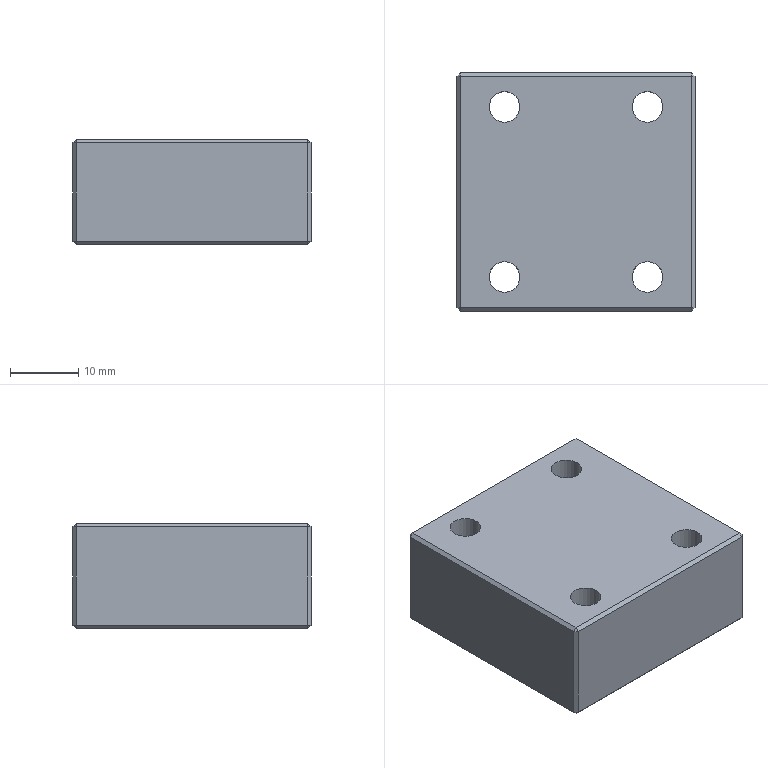Part | NX | 1 solid | 30 faces | box 35 x 35 x 15.5 mm | volume 17959 mm3 | plane 26 | cylinder 4 | commonest cylinder face diameters 4.5 x4
STEP:
#1=CARTESIAN_POINT('',(-17.5,-17.,0.5));
#2=VERTEX_POINT('',#1);
#3=CARTESIAN_POINT('',(-17.5,-17.,15.));
#4=VERTEX_POINT('',#3);
#5=CARTESIAN_POINT('',(-17.5,-17.,15.5));
#6=DIRECTION('',(0.,0.,1.));
#7=VECTOR('',#6,1000.);
#8=LINE('',#5,#7);
#9=EDGE_CURVE('',#2,#4,#8,.T.);
#10=ORIENTED_EDGE('',*,*,#9,.T.);
#11=CARTESIAN_POINT('',(-17.5,17.,15.));
#12=VERTEX_POINT('',#11);
#13=CARTESIAN_POINT('',(-17.5,17.5,15.));
#14=DIRECTION('',(0.,1.,0.));
#15=VECTOR('',#14,1000.);
#16=LINE('',#13,#15);
#17=EDGE_CURVE('',#4,#12,#16,.T.);
#18=ORIENTED_EDGE('',*,*,#17,.T.);
#19=CARTESIAN_POINT('',(-17.5,17.,0.5));
#20=VERTEX_POINT('',#19);
#21=CARTESIAN_POINT('',(-17.5,17.,15.5));
#22=DIRECTION('',(0.,0.,-1.));
#23=VECTOR('',#22,1000.);
#24=LINE('',#21,#23);
#25=EDGE_CURVE('',#12,#20,#24,.T.);
#26=ORIENTED_EDGE('',*,*,#25,.T.);
#27=CARTESIAN_POINT('',(-17.5,-17.5,0.5));
#28=DIRECTION('',(0.,-1.,0.));
#29=VECTOR('',#28,1000.);
#30=LINE('',#27,#29);
#31=EDGE_CURVE('',#20,#2,#30,.T.);
#32=ORIENTED_EDGE('',*,*,#31,.T.);
#33=EDGE_LOOP('',(#10,#18,#26,#32));
#34=FACE_BOUND('',#33,.T.);
#35=CARTESIAN_POINT('',(-17.5,17.5,15.5));
#36=DIRECTION('',(1.,0.,0.));
#37=DIRECTION('',(0.,1.,0.));
#38=AXIS2_PLACEMENT_3D('',#35,#36,#37);
#39=PLANE('',#38);
#40=ADVANCED_FACE('',(#34),#39,.F.);
#41=CARTESIAN_POINT('',(17.,-17.5,15.));
#42=VERTEX_POINT('',#41);
#43=CARTESIAN_POINT('',(-17.,-17.5,15.));
#44=VERTEX_POINT('',#43);
#45=CARTESIAN_POINT('',(17.5,-17.5,15.));
#46=DIRECTION('',(-1.,0.,0.));
#47=VECTOR('',#46,1000.);
#48=LINE('',#45,#47);
#49=EDGE_CURVE('',#42,#44,#48,.T.);
#50=ORIENTED_EDGE('',*,*,#49,.T.);
#51=CARTESIAN_POINT('',(-17.,-17.5,0.5));
#52=VERTEX_POINT('',#51);
#53=CARTESIAN_POINT('',(-17.,-17.5,15.5));
#54=DIRECTION('',(0.,0.,-1.));
#55=VECTOR('',#54,1000.);
#56=LINE('',#53,#55);
#57=EDGE_CURVE('',#44,#52,#56,.T.);
#58=ORIENTED_EDGE('',*,*,#57,.T.);
#59=CARTESIAN_POINT('',(17.,-17.5,0.5));
#60=VERTEX_POINT('',#59);
#61=CARTESIAN_POINT('',(17.5,-17.5,0.5));
#62=DIRECTION('',(1.,0.,0.));
#63=VECTOR('',#62,1000.);
#64=LINE('',#61,#63);
#65=EDGE_CURVE('',#52,#60,#64,.T.);
#66=ORIENTED_EDGE('',*,*,#65,.T.);
#67=CARTESIAN_POINT('',(17.,-17.5,15.5));
#68=DIRECTION('',(0.,0.,1.));
#69=VECTOR('',#68,1000.);
#70=LINE('',#67,#69);
#71=EDGE_CURVE('',#60,#42,#70,.T.);
#72=ORIENTED_EDGE('',*,*,#71,.T.);
#73=EDGE_LOOP('',(#50,#58,#66,#72));
#74=FACE_BOUND('',#73,.T.);
#75=CARTESIAN_POINT('',(17.5,-17.5,15.5));
#76=DIRECTION('',(0.,1.,0.));
#77=DIRECTION('',(-1.,0.,0.));
#78=AXIS2_PLACEMENT_3D('',#75,#76,#77);
#79=PLANE('',#78);
#80=ADVANCED_FACE('',(#74),#79,.F.);
#81=CARTESIAN_POINT('',(17.5,-17.,0.5));
#82=VERTEX_POINT('',#81);
#83=CARTESIAN_POINT('',(17.5,17.,0.5));
#84=VERTEX_POINT('',#83);
#85=CARTESIAN_POINT('',(17.5,17.5,0.5));
#86=DIRECTION('',(0.,1.,0.));
#87=VECTOR('',#86,1000.);
#88=LINE('',#85,#87);
#89=EDGE_CURVE('',#82,#84,#88,.T.);
#90=ORIENTED_EDGE('',*,*,#89,.T.);
#91=CARTESIAN_POINT('',(17.5,17.,15.));
#92=VERTEX_POINT('',#91);
#93=CARTESIAN_POINT('',(17.5,17.,15.5));
#94=DIRECTION('',(0.,0.,1.));
#95=VECTOR('',#94,1000.);
#96=LINE('',#93,#95);
#97=EDGE_CURVE('',#84,#92,#96,.T.);
#98=ORIENTED_EDGE('',*,*,#97,.T.);
#99=CARTESIAN_POINT('',(17.5,-17.,15.));
#100=VERTEX_POINT('',#99);
#101=CARTESIAN_POINT('',(17.5,17.5,15.));
#102=DIRECTION('',(0.,-1.,0.));
#103=VECTOR('',#102,1000.);
#104=LINE('',#101,#103);
#105=EDGE_CURVE('',#92,#100,#104,.T.);
#106=ORIENTED_EDGE('',*,*,#105,.T.);
#107=CARTESIAN_POINT('',(17.5,-17.,15.5));
#108=DIRECTION('',(0.,0.,-1.));
#109=VECTOR('',#108,1000.);
#110=LINE('',#107,#109);
#111=EDGE_CURVE('',#100,#82,#110,.T.);
#112=ORIENTED_EDGE('',*,*,#111,.T.);
#113=EDGE_LOOP('',(#90,#98,#106,#112));
#114=FACE_BOUND('',#113,.T.);
#115=CARTESIAN_POINT('',(17.5,17.5,15.5));
#116=DIRECTION('',(-1.,0.,0.));
#117=DIRECTION('',(0.,-1.,0.));
#118=AXIS2_PLACEMENT_3D('',#115,#116,#117);
#119=PLANE('',#118);
#120=ADVANCED_FACE('',(#114),#119,.F.);
#121=CARTESIAN_POINT('',(-17.,17.5,15.));
#122=VERTEX_POINT('',#121);
#123=CARTESIAN_POINT('',(17.,17.5,15.));
#124=VERTEX_POINT('',#123);
#125=CARTESIAN_POINT('',(17.5,17.5,15.));
#126=DIRECTION('',(1.,0.,0.));
#127=VECTOR('',#126,1000.);
#128=LINE('',#125,#127);
#129=EDGE_CURVE('',#122,#124,#128,.T.);
#130=ORIENTED_EDGE('',*,*,#129,.T.);
#131=CARTESIAN_POINT('',(17.,17.5,0.5));
#132=VERTEX_POINT('',#131);
#133=CARTESIAN_POINT('',(17.,17.5,15.5));
#134=DIRECTION('',(0.,0.,-1.));
#135=VECTOR('',#134,1000.);
#136=LINE('',#133,#135);
#137=EDGE_CURVE('',#124,#132,#136,.T.);
#138=ORIENTED_EDGE('',*,*,#137,.T.);
#139=CARTESIAN_POINT('',(-17.,17.5,0.5));
#140=VERTEX_POINT('',#139);
#141=CARTESIAN_POINT('',(-17.5,17.5,0.5));
#142=DIRECTION('',(-1.,0.,0.));
#143=VECTOR('',#142,1000.);
#144=LINE('',#141,#143);
#145=EDGE_CURVE('',#132,#140,#144,.T.);
#146=ORIENTED_EDGE('',*,*,#145,.T.);
#147=CARTESIAN_POINT('',(-17.,17.5,15.5));
#148=DIRECTION('',(0.,0.,1.));
#149=VECTOR('',#148,1000.);
#150=LINE('',#147,#149);
#151=EDGE_CURVE('',#140,#122,#150,.T.);
#152=ORIENTED_EDGE('',*,*,#151,.T.);
#153=EDGE_LOOP('',(#130,#138,#146,#152));
#154=FACE_BOUND('',#153,.T.);
#155=CARTESIAN_POINT('',(17.5,17.5,15.5));
#156=DIRECTION('',(0.,-1.,0.));
#157=DIRECTION('',(1.,0.,0.));
#158=AXIS2_PLACEMENT_3D('',#155,#156,#157);
#159=PLANE('',#158);
#160=ADVANCED_FACE('',(#154),#159,.F.);
#161=CARTESIAN_POINT('',(17.,-17.,15.5));
#162=VERTEX_POINT('',#161);
#163=CARTESIAN_POINT('',(17.,17.,15.5));
#164=VERTEX_POINT('',#163);
#165=CARTESIAN_POINT('',(17.,0.,15.5));
#166=DIRECTION('',(0.,1.,0.));
#167=VECTOR('',#166,1000.);
#168=LINE('',#165,#167);
#169=EDGE_CURVE('',#162,#164,#168,.T.);
#170=ORIENTED_EDGE('',*,*,#169,.T.);
#171=CARTESIAN_POINT('',(-17.,17.,15.5));
#172=VERTEX_POINT('',#171);
#173=CARTESIAN_POINT('',(0.,17.,15.5));
#174=DIRECTION('',(-1.,0.,0.));
#175=VECTOR('',#174,1000.);
#176=LINE('',#173,#175);
#177=EDGE_CURVE('',#164,#172,#176,.T.);
#178=ORIENTED_EDGE('',*,*,#177,.T.);
#179=CARTESIAN_POINT('',(-17.,-17.,15.5));
#180=VERTEX_POINT('',#179);
#181=CARTESIAN_POINT('',(-17.,0.,15.5));
#182=DIRECTION('',(0.,-1.,0.));
#183=VECTOR('',#182,1000.);
#184=LINE('',#181,#183);
#185=EDGE_CURVE('',#172,#180,#184,.T.);
#186=ORIENTED_EDGE('',*,*,#185,.T.);
#187=CARTESIAN_POINT('',(0.,-17.,15.5));
#188=DIRECTION('',(1.,0.,0.));
#189=VECTOR('',#188,1000.);
#190=LINE('',#187,#189);
#191=EDGE_CURVE('',#180,#162,#190,.T.);
#192=ORIENTED_EDGE('',*,*,#191,.T.);
#193=EDGE_LOOP('',(#170,#178,#186,#192));
#194=FACE_BOUND('',#193,.T.);
#195=CARTESIAN_POINT('',(8.25,12.5,15.5));
#196=VERTEX_POINT('',#195);
#197=CARTESIAN_POINT('',(10.5,12.5,15.5));
#198=DIRECTION('',(0.,0.,-1.));
#199=DIRECTION('',(-1.,0.,0.));
#200=AXIS2_PLACEMENT_3D('',#197,#198,#199);
#201=CIRCLE('',#200,2.25);
#202=EDGE_CURVE('',#196,#196,#201,.T.);
#203=ORIENTED_EDGE('',*,*,#202,.T.);
#204=EDGE_LOOP('',(#203));
#205=FACE_BOUND('',#204,.T.);
#206=CARTESIAN_POINT('',(-12.75,12.5,15.5));
#207=VERTEX_POINT('',#206);
#208=CARTESIAN_POINT('',(-10.5,12.5,15.5));
#209=DIRECTION('',(0.,0.,-1.));
#210=DIRECTION('',(-1.,0.,0.));
#211=AXIS2_PLACEMENT_3D('',#208,#209,#210);
#212=CIRCLE('',#211,2.25);
#213=EDGE_CURVE('',#207,#207,#212,.T.);
#214=ORIENTED_EDGE('',*,*,#213,.T.);
#215=EDGE_LOOP('',(#214));
#216=FACE_BOUND('',#215,.T.);
#217=CARTESIAN_POINT('',(-12.75,-12.5,15.5));
#218=VERTEX_POINT('',#217);
#219=CARTESIAN_POINT('',(-10.5,-12.5,15.5));
#220=DIRECTION('',(0.,0.,-1.));
#221=DIRECTION('',(-1.,0.,0.));
#222=AXIS2_PLACEMENT_3D('',#219,#220,#221);
#223=CIRCLE('',#222,2.25);
#224=EDGE_CURVE('',#218,#218,#223,.T.);
#225=ORIENTED_EDGE('',*,*,#224,.T.);
#226=EDGE_LOOP('',(#225));
#227=FACE_BOUND('',#226,.T.);
#228=CARTESIAN_POINT('',(8.25,-12.5,15.5));
#229=VERTEX_POINT('',#228);
#230=CARTESIAN_POINT('',(10.5,-12.5,15.5));
#231=DIRECTION('',(0.,0.,-1.));
#232=DIRECTION('',(-1.,0.,0.));
#233=AXIS2_PLACEMENT_3D('',#230,#231,#232);
#234=CIRCLE('',#233,2.25);
#235=EDGE_CURVE('',#229,#229,#234,.T.);
#236=ORIENTED_EDGE('',*,*,#235,.T.);
#237=EDGE_LOOP('',(#236));
#238=FACE_BOUND('',#237,.T.);
#239=CARTESIAN_POINT('',(0.,0.,15.5));
#240=DIRECTION('',(0.,0.,-1.));
#241=DIRECTION('',(-1.,0.,0.));
#242=AXIS2_PLACEMENT_3D('',#239,#240,#241);
#243=PLANE('',#242);
#244=ADVANCED_FACE('',(#194,#205,#216,#227,#238),#243,.F.);
#245=CARTESIAN_POINT('',(-17.,-17.,0.));
#246=VERTEX_POINT('',#245);
#247=CARTESIAN_POINT('',(-17.,17.,0.));
#248=VERTEX_POINT('',#247);
#249=CARTESIAN_POINT('',(-17.,17.5,0.));
#250=DIRECTION('',(0.,1.,0.));
#251=VECTOR('',#250,1000.);
#252=LINE('',#249,#251);
#253=EDGE_CURVE('',#246,#248,#252,.T.);
#254=ORIENTED_EDGE('',*,*,#253,.T.);
#255=CARTESIAN_POINT('',(17.,17.,0.));
#256=VERTEX_POINT('',#255);
#257=CARTESIAN_POINT('',(17.5,17.,0.));
#258=DIRECTION('',(1.,0.,0.));
#259=VECTOR('',#258,1000.);
#260=LINE('',#257,#259);
#261=EDGE_CURVE('',#248,#256,#260,.T.);
#262=ORIENTED_EDGE('',*,*,#261,.T.);
#263=CARTESIAN_POINT('',(17.,-17.,0.));
#264=VERTEX_POINT('',#263);
#265=CARTESIAN_POINT('',(17.,-17.5,0.));
#266=DIRECTION('',(0.,-1.,0.));
#267=VECTOR('',#266,1000.);
#268=LINE('',#265,#267);
#269=EDGE_CURVE('',#256,#264,#268,.T.);
#270=ORIENTED_EDGE('',*,*,#269,.T.);
#271=CARTESIAN_POINT('',(-17.5,-17.,0.));
#272=DIRECTION('',(-1.,0.,0.));
#273=VECTOR('',#272,1000.);
#274=LINE('',#271,#273);
#275=EDGE_CURVE('',#264,#246,#274,.T.);
#276=ORIENTED_EDGE('',*,*,#275,.T.);
#277=EDGE_LOOP('',(#254,#262,#270,#276));
#278=FACE_BOUND('',#277,.T.);
#279=CARTESIAN_POINT('',(8.25,12.5,0.));
#280=VERTEX_POINT('',#279);
#281=CARTESIAN_POINT('',(10.5,12.5,0.));
#282=DIRECTION('',(0.,0.,-1.));
#283=DIRECTION('',(-1.,0.,0.));
#284=AXIS2_PLACEMENT_3D('',#281,#282,#283);
#285=CIRCLE('',#284,2.25);
#286=EDGE_CURVE('',#280,#280,#285,.T.);
#287=ORIENTED_EDGE('',*,*,#286,.F.);
#288=EDGE_LOOP('',(#287));
#289=FACE_BOUND('',#288,.T.);
#290=CARTESIAN_POINT('',(-12.75,12.5,0.));
#291=VERTEX_POINT('',#290);
#292=CARTESIAN_POINT('',(-10.5,12.5,0.));
#293=DIRECTION('',(0.,0.,-1.));
#294=DIRECTION('',(-1.,0.,0.));
#295=AXIS2_PLACEMENT_3D('',#292,#293,#294);
#296=CIRCLE('',#295,2.25);
#297=EDGE_CURVE('',#291,#291,#296,.T.);
#298=ORIENTED_EDGE('',*,*,#297,.F.);
#299=EDGE_LOOP('',(#298));
#300=FACE_BOUND('',#299,.T.);
#301=CARTESIAN_POINT('',(-12.75,-12.5,0.));
#302=VERTEX_POINT('',#301);
#303=CARTESIAN_POINT('',(-10.5,-12.5,0.));
#304=DIRECTION('',(0.,0.,-1.));
#305=DIRECTION('',(-1.,0.,0.));
#306=AXIS2_PLACEMENT_3D('',#303,#304,#305);
#307=CIRCLE('',#306,2.25);
#308=EDGE_CURVE('',#302,#302,#307,.T.);
#309=ORIENTED_EDGE('',*,*,#308,.F.);
#310=EDGE_LOOP('',(#309));
#311=FACE_BOUND('',#310,.T.);
#312=CARTESIAN_POINT('',(8.25,-12.5,0.));
#313=VERTEX_POINT('',#312);
#314=CARTESIAN_POINT('',(10.5,-12.5,0.));
#315=DIRECTION('',(0.,0.,-1.));
#316=DIRECTION('',(-1.,0.,0.));
#317=AXIS2_PLACEMENT_3D('',#314,#315,#316);
#318=CIRCLE('',#317,2.25);
#319=EDGE_CURVE('',#313,#313,#318,.T.);
#320=ORIENTED_EDGE('',*,*,#319,.F.);
#321=EDGE_LOOP('',(#320));
#322=FACE_BOUND('',#321,.T.);
#323=CARTESIAN_POINT('',(0.,0.,0.));
#324=DIRECTION('',(0.,0.,-1.));
#325=DIRECTION('',(-1.,0.,0.));
#326=AXIS2_PLACEMENT_3D('',#323,#324,#325);
#327=PLANE('',#326);
#328=ADVANCED_FACE('',(#278,#289,#300,#311,#322),#327,.T.);
#329=ORIENTED_EDGE('',*,*,#235,.F.);
#330=EDGE_LOOP('',(#329));
#331=FACE_BOUND('',#330,.T.);
#332=ORIENTED_EDGE('',*,*,#319,.T.);
#333=EDGE_LOOP('',(#332));
#334=FACE_BOUND('',#333,.T.);
#335=CARTESIAN_POINT('',(10.5,-12.5,0.));
#336=DIRECTION('',(0.,0.,-1.));
#337=DIRECTION('',(-1.,0.,0.));
#338=AXIS2_PLACEMENT_3D('',#335,#336,#337);
#339=CYLINDRICAL_SURFACE('',#338,2.25);
#340=ADVANCED_FACE('',(#331,#334),#339,.F.);
#341=ORIENTED_EDGE('',*,*,#224,.F.);
#342=EDGE_LOOP('',(#341));
#343=FACE_BOUND('',#342,.T.);
#344=ORIENTED_EDGE('',*,*,#308,.T.);
#345=EDGE_LOOP('',(#344));
#346=FACE_BOUND('',#345,.T.);
#347=CARTESIAN_POINT('',(-10.5,-12.5,0.));
#348=DIRECTION('',(0.,0.,-1.));
#349=DIRECTION('',(-1.,0.,0.));
#350=AXIS2_PLACEMENT_3D('',#347,#348,#349);
#351=CYLINDRICAL_SURFACE('',#350,2.25);
#352=ADVANCED_FACE('',(#343,#346),#351,.F.);
#353=ORIENTED_EDGE('',*,*,#213,.F.);
#354=EDGE_LOOP('',(#353));
#355=FACE_BOUND('',#354,.T.);
#356=ORIENTED_EDGE('',*,*,#297,.T.);
#357=EDGE_LOOP('',(#356));
#358=FACE_BOUND('',#357,.T.);
#359=CARTESIAN_POINT('',(-10.5,12.5,0.));
#360=DIRECTION('',(0.,0.,-1.));
#361=DIRECTION('',(-1.,0.,0.));
#362=AXIS2_PLACEMENT_3D('',#359,#360,#361);
#363=CYLINDRICAL_SURFACE('',#362,2.25);
#364=ADVANCED_FACE('',(#355,#358),#363,.F.);
#365=ORIENTED_EDGE('',*,*,#202,.F.);
#366=EDGE_LOOP('',(#365));
#367=FACE_BOUND('',#366,.T.);
#368=ORIENTED_EDGE('',*,*,#286,.T.);
#369=EDGE_LOOP('',(#368));
#370=FACE_BOUND('',#369,.T.);
#371=CARTESIAN_POINT('',(10.5,12.5,0.));
#372=DIRECTION('',(0.,0.,-1.));
#373=DIRECTION('',(-1.,0.,0.));
#374=AXIS2_PLACEMENT_3D('',#371,#372,#373);
#375=CYLINDRICAL_SURFACE('',#374,2.25);
#376=ADVANCED_FACE('',(#367,#370),#375,.F.);
#377=CARTESIAN_POINT('',(-17.5,-17.,15.));
#378=DIRECTION('',(-0.7071,0.7071,0.));
#379=VECTOR('',#378,1000.);
#380=LINE('',#377,#379);
#381=EDGE_CURVE('',#4,#44,#380,.F.);
#382=ORIENTED_EDGE('',*,*,#381,.F.);
#383=ORIENTED_EDGE('',*,*,#9,.F.);
#384=CARTESIAN_POINT('',(-17.,-17.5,0.5));
#385=DIRECTION('',(0.7071,-0.7071,0.));
#386=VECTOR('',#385,1000.);
#387=LINE('',#384,#386);
#388=EDGE_CURVE('',#52,#2,#387,.F.);
#389=ORIENTED_EDGE('',*,*,#388,.F.);
#390=ORIENTED_EDGE('',*,*,#57,.F.);
#391=EDGE_LOOP('',(#382,#383,#389,#390));
#392=FACE_BOUND('',#391,.T.);
#393=CARTESIAN_POINT('',(-17.,-17.5,15.5));
#394=DIRECTION('',(0.7071,0.7071,0.));
#395=DIRECTION('',(0.,0.,-1.));
#396=AXIS2_PLACEMENT_3D('',#393,#394,#395);
#397=PLANE('',#396);
#398=ADVANCED_FACE('',(#392),#397,.F.);
#399=CARTESIAN_POINT('',(-17.5,-17.,15.));
#400=DIRECTION('',(0.7071,0.,0.7071));
#401=VECTOR('',#400,1000.);
#402=LINE('',#399,#401);
#403=EDGE_CURVE('',#4,#180,#402,.T.);
#404=ORIENTED_EDGE('',*,*,#403,.F.);
#405=ORIENTED_EDGE('',*,*,#381,.T.);
#406=CARTESIAN_POINT('',(-17.,-17.25,15.25));
#407=DIRECTION('',(0.,-0.7071,-0.7071));
#408=VECTOR('',#407,1000.);
#409=LINE('',#406,#408);
#410=EDGE_CURVE('',#180,#44,#409,.T.);
#411=ORIENTED_EDGE('',*,*,#410,.F.);
#412=EDGE_LOOP('',(#404,#405,#411));
#413=FACE_BOUND('',#412,.T.);
#414=CARTESIAN_POINT('',(-17.5,-17.,15.));
#415=DIRECTION('',(-0.5774,-0.5774,0.5774));
#416=DIRECTION('',(0.7071,0.,0.7071));
#417=AXIS2_PLACEMENT_3D('',#414,#415,#416);
#418=PLANE('',#417);
#419=ADVANCED_FACE('',(#413),#418,.T.);
#420=CARTESIAN_POINT('',(-17.,-17.5,0.5));
#421=DIRECTION('',(0.,-0.7071,0.7071));
#422=VECTOR('',#421,1000.);
#423=LINE('',#420,#422);
#424=EDGE_CURVE('',#52,#246,#423,.F.);
#425=ORIENTED_EDGE('',*,*,#424,.F.);
#426=ORIENTED_EDGE('',*,*,#388,.T.);
#427=CARTESIAN_POINT('',(-17.25,-17.,0.25));
#428=DIRECTION('',(0.7071,0.,-0.7071));
#429=VECTOR('',#428,1000.);
#430=LINE('',#427,#429);
#431=EDGE_CURVE('',#246,#2,#430,.F.);
#432=ORIENTED_EDGE('',*,*,#431,.F.);
#433=EDGE_LOOP('',(#425,#426,#432));
#434=FACE_BOUND('',#433,.T.);
#435=CARTESIAN_POINT('',(-17.,-17.5,0.5));
#436=DIRECTION('',(-0.5774,-0.5774,-0.5774));
#437=DIRECTION('',(-0.7071,0.,0.7071));
#438=AXIS2_PLACEMENT_3D('',#435,#436,#437);
#439=PLANE('',#438);
#440=ADVANCED_FACE('',(#434),#439,.T.);
#441=ORIENTED_EDGE('',*,*,#410,.T.);
#442=ORIENTED_EDGE('',*,*,#49,.F.);
#443=CARTESIAN_POINT('',(17.,-17.,15.5));
#444=DIRECTION('',(0.,0.7071,0.7071));
#445=VECTOR('',#444,1000.);
#446=LINE('',#443,#445);
#447=EDGE_CURVE('',#162,#42,#446,.F.);
#448=ORIENTED_EDGE('',*,*,#447,.F.);
#449=ORIENTED_EDGE('',*,*,#191,.F.);
#450=EDGE_LOOP('',(#441,#442,#448,#449));
#451=FACE_BOUND('',#450,.T.);
#452=CARTESIAN_POINT('',(0.,-17.,15.5));
#453=DIRECTION('',(0.,0.7071,-0.7071));
#454=DIRECTION('',(1.,0.,0.));
#455=AXIS2_PLACEMENT_3D('',#452,#453,#454);
#456=PLANE('',#455);
#457=ADVANCED_FACE('',(#451),#456,.F.);
#458=ORIENTED_EDGE('',*,*,#403,.T.);
#459=ORIENTED_EDGE('',*,*,#185,.F.);
#460=CARTESIAN_POINT('',(-17.,17.,15.5));
#461=DIRECTION('',(-0.7071,0.,-0.7071));
#462=VECTOR('',#461,1000.);
#463=LINE('',#460,#462);
#464=EDGE_CURVE('',#12,#172,#463,.F.);
#465=ORIENTED_EDGE('',*,*,#464,.F.);
#466=ORIENTED_EDGE('',*,*,#17,.F.);
#467=EDGE_LOOP('',(#458,#459,#465,#466));
#468=FACE_BOUND('',#467,.T.);
#469=CARTESIAN_POINT('',(-17.,0.,15.5));
#470=DIRECTION('',(0.7071,0.,-0.7071));
#471=DIRECTION('',(0.,-1.,0.));
#472=AXIS2_PLACEMENT_3D('',#469,#470,#471);
#473=PLANE('',#472);
#474=ADVANCED_FACE('',(#468),#473,.F.);
#475=CARTESIAN_POINT('',(-17.5,17.,0.5));
#476=DIRECTION('',(-0.7071,-0.7071,0.));
#477=VECTOR('',#476,1000.);
#478=LINE('',#475,#477);
#479=EDGE_CURVE('',#20,#140,#478,.F.);
#480=ORIENTED_EDGE('',*,*,#479,.F.);
#481=ORIENTED_EDGE('',*,*,#25,.F.);
#482=CARTESIAN_POINT('',(-17.25,17.25,15.));
#483=DIRECTION('',(0.7071,0.7071,0.));
#484=VECTOR('',#483,1000.);
#485=LINE('',#482,#484);
#486=EDGE_CURVE('',#122,#12,#485,.F.);
#487=ORIENTED_EDGE('',*,*,#486,.F.);
#488=ORIENTED_EDGE('',*,*,#151,.F.);
#489=EDGE_LOOP('',(#480,#481,#487,#488));
#490=FACE_BOUND('',#489,.T.);
#491=CARTESIAN_POINT('',(-17.5,17.,15.5));
#492=DIRECTION('',(0.7071,-0.7071,0.));
#493=DIRECTION('',(0.,0.,-1.));
#494=AXIS2_PLACEMENT_3D('',#491,#492,#493);
#495=PLANE('',#494);
#496=ADVANCED_FACE('',(#490),#495,.F.);
#497=ORIENTED_EDGE('',*,*,#431,.T.);
#498=ORIENTED_EDGE('',*,*,#31,.F.);
#499=CARTESIAN_POINT('',(-17.5,17.,0.5));
#500=DIRECTION('',(-0.7071,0.,0.7071));
#501=VECTOR('',#500,1000.);
#502=LINE('',#499,#501);
#503=EDGE_CURVE('',#248,#20,#502,.T.);
#504=ORIENTED_EDGE('',*,*,#503,.F.);
#505=ORIENTED_EDGE('',*,*,#253,.F.);
#506=EDGE_LOOP('',(#497,#498,#504,#505));
#507=FACE_BOUND('',#506,.T.);
#508=CARTESIAN_POINT('',(-17.5,17.5,0.5));
#509=DIRECTION('',(-0.7071,0.,-0.7071));
#510=DIRECTION('',(0.,1.,0.));
#511=AXIS2_PLACEMENT_3D('',#508,#509,#510);
#512=PLANE('',#511);
#513=ADVANCED_FACE('',(#507),#512,.T.);
#514=ORIENTED_EDGE('',*,*,#424,.T.);
#515=ORIENTED_EDGE('',*,*,#275,.F.);
#516=CARTESIAN_POINT('',(17.,-17.25,0.25));
#517=DIRECTION('',(0.,0.7071,-0.7071));
#518=VECTOR('',#517,1000.);
#519=LINE('',#516,#518);
#520=EDGE_CURVE('',#60,#264,#519,.T.);
#521=ORIENTED_EDGE('',*,*,#520,.F.);
#522=ORIENTED_EDGE('',*,*,#65,.F.);
#523=EDGE_LOOP('',(#514,#515,#521,#522));
#524=FACE_BOUND('',#523,.T.);
#525=CARTESIAN_POINT('',(17.5,-17.5,0.5));
#526=DIRECTION('',(0.,-0.7071,-0.7071));
#527=DIRECTION('',(-1.,0.,0.));
#528=AXIS2_PLACEMENT_3D('',#525,#526,#527);
#529=PLANE('',#528);
#530=ADVANCED_FACE('',(#524),#529,.T.);
#531=CARTESIAN_POINT('',(17.25,-17.25,15.));
#532=DIRECTION('',(-0.7071,-0.7071,0.));
#533=VECTOR('',#532,1000.);
#534=LINE('',#531,#533);
#535=EDGE_CURVE('',#42,#100,#534,.F.);
#536=ORIENTED_EDGE('',*,*,#535,.F.);
#537=ORIENTED_EDGE('',*,*,#71,.F.);
#538=CARTESIAN_POINT('',(17.5,-17.,0.5));
#539=DIRECTION('',(0.7071,0.7071,0.));
#540=VECTOR('',#539,1000.);
#541=LINE('',#538,#540);
#542=EDGE_CURVE('',#82,#60,#541,.F.);
#543=ORIENTED_EDGE('',*,*,#542,.F.);
#544=ORIENTED_EDGE('',*,*,#111,.F.);
#545=EDGE_LOOP('',(#536,#537,#543,#544));
#546=FACE_BOUND('',#545,.T.);
#547=CARTESIAN_POINT('',(17.5,-17.,15.5));
#548=DIRECTION('',(-0.7071,0.7071,0.));
#549=DIRECTION('',(0.,0.,-1.));
#550=AXIS2_PLACEMENT_3D('',#547,#548,#549);
#551=PLANE('',#550);
#552=ADVANCED_FACE('',(#546),#551,.F.);
#553=ORIENTED_EDGE('',*,*,#447,.T.);
#554=ORIENTED_EDGE('',*,*,#535,.T.);
#555=CARTESIAN_POINT('',(17.,-17.,15.5));
#556=DIRECTION('',(0.7071,0.,-0.7071));
#557=VECTOR('',#556,1000.);
#558=LINE('',#555,#557);
#559=EDGE_CURVE('',#162,#100,#558,.T.);
#560=ORIENTED_EDGE('',*,*,#559,.F.);
#561=EDGE_LOOP('',(#553,#554,#560));
#562=FACE_BOUND('',#561,.T.);
#563=CARTESIAN_POINT('',(17.,-17.,15.5));
#564=DIRECTION('',(0.5774,-0.5774,0.5774));
#565=DIRECTION('',(0.7071,0.,-0.7071));
#566=AXIS2_PLACEMENT_3D('',#563,#564,#565);
#567=PLANE('',#566);
#568=ADVANCED_FACE('',(#562),#567,.T.);
#569=ORIENTED_EDGE('',*,*,#486,.T.);
#570=ORIENTED_EDGE('',*,*,#464,.T.);
#571=CARTESIAN_POINT('',(-17.,17.,15.5));
#572=DIRECTION('',(0.,-0.7071,0.7071));
#573=VECTOR('',#572,1000.);
#574=LINE('',#571,#573);
#575=EDGE_CURVE('',#122,#172,#574,.T.);
#576=ORIENTED_EDGE('',*,*,#575,.F.);
#577=EDGE_LOOP('',(#569,#570,#576));
#578=FACE_BOUND('',#577,.T.);
#579=CARTESIAN_POINT('',(-17.,17.,15.5));
#580=DIRECTION('',(-0.5774,0.5774,0.5774));
#581=DIRECTION('',(0.,-0.7071,0.7071));
#582=AXIS2_PLACEMENT_3D('',#579,#580,#581);
#583=PLANE('',#582);
#584=ADVANCED_FACE('',(#578),#583,.T.);
#585=ORIENTED_EDGE('',*,*,#503,.T.);
#586=ORIENTED_EDGE('',*,*,#479,.T.);
#587=CARTESIAN_POINT('',(-17.,17.25,0.25));
#588=DIRECTION('',(0.,-0.7071,-0.7071));
#589=VECTOR('',#588,1000.);
#590=LINE('',#587,#589);
#591=EDGE_CURVE('',#248,#140,#590,.F.);
#592=ORIENTED_EDGE('',*,*,#591,.F.);
#593=EDGE_LOOP('',(#585,#586,#592));
#594=FACE_BOUND('',#593,.T.);
#595=CARTESIAN_POINT('',(-17.5,17.,0.5));
#596=DIRECTION('',(-0.5774,0.5774,-0.5774));
#597=DIRECTION('',(0.,0.7071,0.7071));
#598=AXIS2_PLACEMENT_3D('',#595,#596,#597);
#599=PLANE('',#598);
#600=ADVANCED_FACE('',(#594),#599,.T.);
#601=ORIENTED_EDGE('',*,*,#542,.T.);
#602=ORIENTED_EDGE('',*,*,#520,.T.);
#603=CARTESIAN_POINT('',(17.5,-17.,0.5));
#604=DIRECTION('',(0.7071,0.,0.7071));
#605=VECTOR('',#604,1000.);
#606=LINE('',#603,#605);
#607=EDGE_CURVE('',#82,#264,#606,.F.);
#608=ORIENTED_EDGE('',*,*,#607,.F.);
#609=EDGE_LOOP('',(#601,#602,#608));
#610=FACE_BOUND('',#609,.T.);
#611=CARTESIAN_POINT('',(17.5,-17.,0.5));
#612=DIRECTION('',(0.5774,-0.5774,-0.5774));
#613=DIRECTION('',(-0.7071,0.,-0.7071));
#614=AXIS2_PLACEMENT_3D('',#611,#612,#613);
#615=PLANE('',#614);
#616=ADVANCED_FACE('',(#610),#615,.T.);
#617=ORIENTED_EDGE('',*,*,#559,.T.);
#618=ORIENTED_EDGE('',*,*,#105,.F.);
#619=CARTESIAN_POINT('',(17.5,17.,15.));
#620=DIRECTION('',(-0.7071,0.,0.7071));
#621=VECTOR('',#620,1000.);
#622=LINE('',#619,#621);
#623=EDGE_CURVE('',#164,#92,#622,.F.);
#624=ORIENTED_EDGE('',*,*,#623,.F.);
#625=ORIENTED_EDGE('',*,*,#169,.F.);
#626=EDGE_LOOP('',(#617,#618,#624,#625));
#627=FACE_BOUND('',#626,.T.);
#628=CARTESIAN_POINT('',(17.,0.,15.5));
#629=DIRECTION('',(-0.7071,0.,-0.7071));
#630=DIRECTION('',(0.,1.,0.));
#631=AXIS2_PLACEMENT_3D('',#628,#629,#630);
#632=PLANE('',#631);
#633=ADVANCED_FACE('',(#627),#632,.F.);
#634=ORIENTED_EDGE('',*,*,#575,.T.);
#635=ORIENTED_EDGE('',*,*,#177,.F.);
#636=CARTESIAN_POINT('',(17.,17.25,15.25));
#637=DIRECTION('',(0.,0.7071,-0.7071));
#638=VECTOR('',#637,1000.);
#639=LINE('',#636,#638);
#640=EDGE_CURVE('',#124,#164,#639,.F.);
#641=ORIENTED_EDGE('',*,*,#640,.F.);
#642=ORIENTED_EDGE('',*,*,#129,.F.);
#643=EDGE_LOOP('',(#634,#635,#641,#642));
#644=FACE_BOUND('',#643,.T.);
#645=CARTESIAN_POINT('',(0.,17.,15.5));
#646=DIRECTION('',(0.,-0.7071,-0.7071));
#647=DIRECTION('',(-1.,0.,0.));
#648=AXIS2_PLACEMENT_3D('',#645,#646,#647);
#649=PLANE('',#648);
#650=ADVANCED_FACE('',(#644),#649,.F.);
#651=ORIENTED_EDGE('',*,*,#591,.T.);
#652=ORIENTED_EDGE('',*,*,#145,.F.);
#653=CARTESIAN_POINT('',(17.,17.5,0.5));
#654=DIRECTION('',(0.,0.7071,0.7071));
#655=VECTOR('',#654,1000.);
#656=LINE('',#653,#655);
#657=EDGE_CURVE('',#256,#132,#656,.T.);
#658=ORIENTED_EDGE('',*,*,#657,.F.);
#659=ORIENTED_EDGE('',*,*,#261,.F.);
#660=EDGE_LOOP('',(#651,#652,#658,#659));
#661=FACE_BOUND('',#660,.T.);
#662=CARTESIAN_POINT('',(17.5,17.5,0.5));
#663=DIRECTION('',(0.,0.7071,-0.7071));
#664=DIRECTION('',(1.,0.,0.));
#665=AXIS2_PLACEMENT_3D('',#662,#663,#664);
#666=PLANE('',#665);
#667=ADVANCED_FACE('',(#661),#666,.T.);
#668=ORIENTED_EDGE('',*,*,#607,.T.);
#669=ORIENTED_EDGE('',*,*,#269,.F.);
#670=CARTESIAN_POINT('',(17.25,17.,0.25));
#671=DIRECTION('',(-0.7071,0.,-0.7071));
#672=VECTOR('',#671,1000.);
#673=LINE('',#670,#672);
#674=EDGE_CURVE('',#84,#256,#673,.T.);
#675=ORIENTED_EDGE('',*,*,#674,.F.);
#676=ORIENTED_EDGE('',*,*,#89,.F.);
#677=EDGE_LOOP('',(#668,#669,#675,#676));
#678=FACE_BOUND('',#677,.T.);
#679=CARTESIAN_POINT('',(17.5,17.5,0.5));
#680=DIRECTION('',(0.7071,0.,-0.7071));
#681=DIRECTION('',(0.,-1.,0.));
#682=AXIS2_PLACEMENT_3D('',#679,#680,#681);
#683=PLANE('',#682);
#684=ADVANCED_FACE('',(#678),#683,.T.);
#685=ORIENTED_EDGE('',*,*,#640,.T.);
#686=ORIENTED_EDGE('',*,*,#623,.T.);
#687=CARTESIAN_POINT('',(17.5,17.,15.));
#688=DIRECTION('',(0.7071,-0.7071,0.));
#689=VECTOR('',#688,1000.);
#690=LINE('',#687,#689);
#691=EDGE_CURVE('',#124,#92,#690,.T.);
#692=ORIENTED_EDGE('',*,*,#691,.F.);
#693=EDGE_LOOP('',(#685,#686,#692));
#694=FACE_BOUND('',#693,.T.);
#695=CARTESIAN_POINT('',(17.5,17.,15.));
#696=DIRECTION('',(0.5774,0.5774,0.5774));
#697=DIRECTION('',(0.7071,0.,-0.7071));
#698=AXIS2_PLACEMENT_3D('',#695,#696,#697);
#699=PLANE('',#698);
#700=ADVANCED_FACE('',(#694),#699,.T.);
#701=ORIENTED_EDGE('',*,*,#674,.T.);
#702=ORIENTED_EDGE('',*,*,#657,.T.);
#703=CARTESIAN_POINT('',(17.,17.5,0.5));
#704=DIRECTION('',(-0.7071,0.7071,0.));
#705=VECTOR('',#704,1000.);
#706=LINE('',#703,#705);
#707=EDGE_CURVE('',#84,#132,#706,.T.);
#708=ORIENTED_EDGE('',*,*,#707,.F.);
#709=EDGE_LOOP('',(#701,#702,#708));
#710=FACE_BOUND('',#709,.T.);
#711=CARTESIAN_POINT('',(17.,17.5,0.5));
#712=DIRECTION('',(0.5774,0.5774,-0.5774));
#713=DIRECTION('',(-0.7071,0.,-0.7071));
#714=AXIS2_PLACEMENT_3D('',#711,#712,#713);
#715=PLANE('',#714);
#716=ADVANCED_FACE('',(#710),#715,.T.);
#717=ORIENTED_EDGE('',*,*,#691,.T.);
#718=ORIENTED_EDGE('',*,*,#97,.F.);
#719=ORIENTED_EDGE('',*,*,#707,.T.);
#720=ORIENTED_EDGE('',*,*,#137,.F.);
#721=EDGE_LOOP('',(#717,#718,#719,#720));
#722=FACE_BOUND('',#721,.T.);
#723=CARTESIAN_POINT('',(17.,17.5,15.5));
#724=DIRECTION('',(-0.7071,-0.7071,0.));
#725=DIRECTION('',(0.,0.,-1.));
#726=AXIS2_PLACEMENT_3D('',#723,#724,#725);
#727=PLANE('',#726);
#728=ADVANCED_FACE('',(#722),#727,.F.);
#729=CLOSED_SHELL('',(#40,#80,#120,#160,#244,#328,#340,#352,#364,#376,#398,#419,#440,#457,#474,#496,#513,#530,#552,#568,#584,#600,#616,#633,#650,#667,#684,#700,#716,#728));
#730=MANIFOLD_SOLID_BREP('',#729);
#731=(LENGTH_UNIT()NAMED_UNIT(*)SI_UNIT(.MILLI.,.METRE.));
#732=UNCERTAINTY_MEASURE_WITH_UNIT(LENGTH_MEASURE(0.00001),#731,'','');
#733=(NAMED_UNIT(*)PLANE_ANGLE_UNIT()SI_UNIT($,.RADIAN.));
#734=(NAMED_UNIT(*)SI_UNIT($,.STERADIAN.)SOLID_ANGLE_UNIT());
#735=(GEOMETRIC_REPRESENTATION_CONTEXT(3)GLOBAL_UNCERTAINTY_ASSIGNED_CONTEXT((#732))GLOBAL_UNIT_ASSIGNED_CONTEXT((#731,#733,#734))REPRESENTATION_CONTEXT('',''));
#736=ADVANCED_BREP_SHAPE_REPRESENTATION('',(#730),#735);